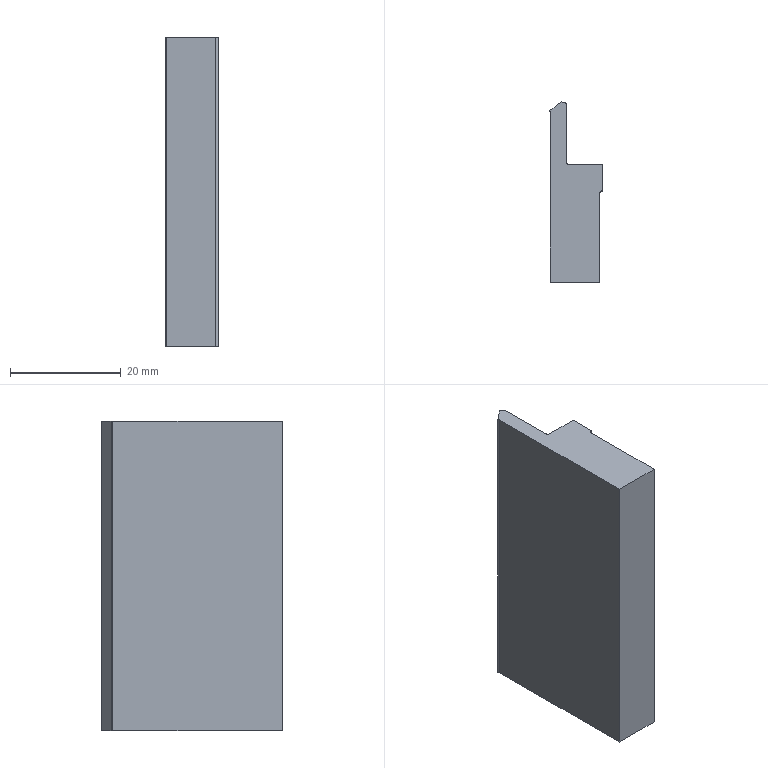Part | NX | features BREP 2 | 2 solids | 28 faces | box 9.487 x 32.71 x 56 mm | volume 24904 mm3 | plane 18 | cylinder 10 | commonest cylinder face diameters 1 x10
STEP:
#1=CARTESIAN_POINT('',(4.221,-0.3316,-4.));
#2=VERTEX_POINT('',#1);
#3=CARTESIAN_POINT('',(4.221,-0.3316,52.));
#4=VERTEX_POINT('',#3);
#5=CARTESIAN_POINT('',(4.221,-0.3316,0.));
#6=DIRECTION('',(0.,0.,1.));
#7=VECTOR('',#6,1000.);
#8=LINE('',#5,#7);
#9=EDGE_CURVE('',#2,#4,#8,.T.);
#10=ORIENTED_EDGE('',*,*,#9,.T.);
#11=CARTESIAN_POINT('',(4.221,-16.355,52.));
#12=VERTEX_POINT('',#11);
#13=CARTESIAN_POINT('',(4.221,10.146,52.));
#14=DIRECTION('',(0.,1.,0.));
#15=VECTOR('',#14,1000.);
#16=LINE('',#13,#15);
#17=EDGE_CURVE('',#12,#4,#16,.T.);
#18=ORIENTED_EDGE('',*,*,#17,.F.);
#19=CARTESIAN_POINT('',(4.221,-16.355,-4.));
#20=VERTEX_POINT('',#19);
#21=CARTESIAN_POINT('',(4.221,-16.355,0.));
#22=DIRECTION('',(0.,0.,1.));
#23=VECTOR('',#22,1000.);
#24=LINE('',#21,#23);
#25=EDGE_CURVE('',#20,#12,#24,.T.);
#26=ORIENTED_EDGE('',*,*,#25,.F.);
#27=CARTESIAN_POINT('',(4.221,10.146,-4.));
#28=DIRECTION('',(0.,1.,0.));
#29=VECTOR('',#28,1000.);
#30=LINE('',#27,#29);
#31=EDGE_CURVE('',#20,#2,#30,.T.);
#32=ORIENTED_EDGE('',*,*,#31,.T.);
#33=EDGE_LOOP('',(#10,#18,#26,#32));
#34=FACE_BOUND('',#33,.T.);
#35=CARTESIAN_POINT('',(4.221,-0.3316,0.));
#36=DIRECTION('',(-1.,0.,0.));
#37=DIRECTION('',(0.,1.,0.));
#38=AXIS2_PLACEMENT_3D('',#35,#36,#37);
#39=PLANE('',#38);
#40=ADVANCED_FACE('',(#34),#39,.F.);
#41=ORIENTED_EDGE('',*,*,#25,.T.);
#42=CARTESIAN_POINT('',(-4.656,-16.355,52.));
#43=VERTEX_POINT('',#42);
#44=CARTESIAN_POINT('',(13.794,-16.355,52.));
#45=DIRECTION('',(1.,0.,0.));
#46=VECTOR('',#45,1000.);
#47=LINE('',#44,#46);
#48=EDGE_CURVE('',#43,#12,#47,.T.);
#49=ORIENTED_EDGE('',*,*,#48,.F.);
#50=CARTESIAN_POINT('',(-4.656,-16.355,-4.));
#51=VERTEX_POINT('',#50);
#52=CARTESIAN_POINT('',(-4.656,-16.355,0.));
#53=DIRECTION('',(0.,0.,1.));
#54=VECTOR('',#53,1000.);
#55=LINE('',#52,#54);
#56=EDGE_CURVE('',#51,#43,#55,.T.);
#57=ORIENTED_EDGE('',*,*,#56,.F.);
#58=CARTESIAN_POINT('',(13.794,-16.355,-4.));
#59=DIRECTION('',(1.,0.,0.));
#60=VECTOR('',#59,1000.);
#61=LINE('',#58,#60);
#62=EDGE_CURVE('',#51,#20,#61,.T.);
#63=ORIENTED_EDGE('',*,*,#62,.T.);
#64=EDGE_LOOP('',(#41,#49,#57,#63));
#65=FACE_BOUND('',#64,.T.);
#66=CARTESIAN_POINT('',(-4.656,-16.355,0.));
#67=DIRECTION('',(0.,-1.,0.));
#68=DIRECTION('',(-1.,0.,0.));
#69=AXIS2_PLACEMENT_3D('',#66,#67,#68);
#70=PLANE('',#69);
#71=ADVANCED_FACE('',(#65),#70,.T.);
#72=ORIENTED_EDGE('',*,*,#56,.T.);
#73=CARTESIAN_POINT('',(-4.656,14.338,52.));
#74=VERTEX_POINT('',#73);
#75=CARTESIAN_POINT('',(-4.656,10.146,52.));
#76=DIRECTION('',(0.,-1.,0.));
#77=VECTOR('',#76,1000.);
#78=LINE('',#75,#77);
#79=EDGE_CURVE('',#74,#43,#78,.T.);
#80=ORIENTED_EDGE('',*,*,#79,.F.);
#81=CARTESIAN_POINT('',(-4.656,14.338,-4.));
#82=VERTEX_POINT('',#81);
#83=CARTESIAN_POINT('',(-4.656,14.338,0.));
#84=DIRECTION('',(0.,0.,1.));
#85=VECTOR('',#84,1000.);
#86=LINE('',#83,#85);
#87=EDGE_CURVE('',#82,#74,#86,.T.);
#88=ORIENTED_EDGE('',*,*,#87,.F.);
#89=CARTESIAN_POINT('',(-4.656,10.146,-4.));
#90=DIRECTION('',(0.,-1.,0.));
#91=VECTOR('',#90,1000.);
#92=LINE('',#89,#91);
#93=EDGE_CURVE('',#82,#51,#92,.T.);
#94=ORIENTED_EDGE('',*,*,#93,.T.);
#95=EDGE_LOOP('',(#72,#80,#88,#94));
#96=FACE_BOUND('',#95,.T.);
#97=CARTESIAN_POINT('',(-4.656,-17.855,0.));
#98=DIRECTION('',(1.,0.,0.));
#99=DIRECTION('',(0.,-1.,0.));
#100=AXIS2_PLACEMENT_3D('',#97,#98,#99);
#101=PLANE('',#100);
#102=ADVANCED_FACE('',(#96),#101,.F.);
#103=ORIENTED_EDGE('',*,*,#87,.T.);
#104=CARTESIAN_POINT('',(-4.766,14.651,52.));
#105=VERTEX_POINT('',#104);
#106=CARTESIAN_POINT('',(-5.156,14.338,52.));
#107=DIRECTION('',(0.,0.,-1.));
#108=DIRECTION('',(1.,0.,0.));
#109=AXIS2_PLACEMENT_3D('',#106,#107,#108);
#110=CIRCLE('',#109,0.5);
#111=EDGE_CURVE('',#105,#74,#110,.T.);
#112=ORIENTED_EDGE('',*,*,#111,.F.);
#113=CARTESIAN_POINT('',(-4.766,14.651,-4.));
#114=VERTEX_POINT('',#113);
#115=CARTESIAN_POINT('',(-4.766,14.651,0.));
#116=DIRECTION('',(0.,0.,1.));
#117=VECTOR('',#116,1000.);
#118=LINE('',#115,#117);
#119=EDGE_CURVE('',#114,#105,#118,.T.);
#120=ORIENTED_EDGE('',*,*,#119,.F.);
#121=CARTESIAN_POINT('',(-5.156,14.338,-4.));
#122=DIRECTION('',(0.,0.,-1.));
#123=DIRECTION('',(1.,0.,0.));
#124=AXIS2_PLACEMENT_3D('',#121,#122,#123);
#125=CIRCLE('',#124,0.5);
#126=EDGE_CURVE('',#114,#82,#125,.T.);
#127=ORIENTED_EDGE('',*,*,#126,.T.);
#128=EDGE_LOOP('',(#103,#112,#120,#127));
#129=FACE_BOUND('',#128,.T.);
#130=CARTESIAN_POINT('',(-5.156,14.338,0.));
#131=DIRECTION('',(0.,0.,1.));
#132=DIRECTION('',(-1.,0.,0.));
#133=AXIS2_PLACEMENT_3D('',#130,#131,#132);
#134=CYLINDRICAL_SURFACE('',#133,0.5);
#135=ADVANCED_FACE('',(#129),#134,.F.);
#136=ORIENTED_EDGE('',*,*,#119,.T.);
#137=CARTESIAN_POINT('',(-2.645,16.355,52.));
#138=VERTEX_POINT('',#137);
#139=CARTESIAN_POINT('',(-5.156,14.338,52.));
#140=DIRECTION('',(-0.7795,-0.6264,0.));
#141=VECTOR('',#140,1000.);
#142=LINE('',#139,#141);
#143=EDGE_CURVE('',#138,#105,#142,.T.);
#144=ORIENTED_EDGE('',*,*,#143,.F.);
#145=CARTESIAN_POINT('',(-2.645,16.355,-4.));
#146=VERTEX_POINT('',#145);
#147=CARTESIAN_POINT('',(-2.645,16.355,0.));
#148=DIRECTION('',(0.,0.,1.));
#149=VECTOR('',#148,1000.);
#150=LINE('',#147,#149);
#151=EDGE_CURVE('',#146,#138,#150,.T.);
#152=ORIENTED_EDGE('',*,*,#151,.F.);
#153=CARTESIAN_POINT('',(-5.156,14.338,-4.));
#154=DIRECTION('',(-0.7795,-0.6264,0.));
#155=VECTOR('',#154,1000.);
#156=LINE('',#153,#155);
#157=EDGE_CURVE('',#146,#114,#156,.T.);
#158=ORIENTED_EDGE('',*,*,#157,.T.);
#159=EDGE_LOOP('',(#136,#144,#152,#158));
#160=FACE_BOUND('',#159,.T.);
#161=CARTESIAN_POINT('',(-5.156,14.338,0.));
#162=DIRECTION('',(0.6264,-0.7795,0.));
#163=DIRECTION('',(-0.7795,-0.6264,0.));
#164=AXIS2_PLACEMENT_3D('',#161,#162,#163);
#165=PLANE('',#164);
#166=ADVANCED_FACE('',(#160),#165,.F.);
#167=ORIENTED_EDGE('',*,*,#151,.T.);
#168=CARTESIAN_POINT('',(-2.256,16.168,52.));
#169=VERTEX_POINT('',#168);
#170=CARTESIAN_POINT('',(-2.256,16.668,52.));
#171=DIRECTION('',(0.,0.,-1.));
#172=DIRECTION('',(1.,0.,0.));
#173=AXIS2_PLACEMENT_3D('',#170,#171,#172);
#174=CIRCLE('',#173,0.5);
#175=EDGE_CURVE('',#169,#138,#174,.T.);
#176=ORIENTED_EDGE('',*,*,#175,.F.);
#177=CARTESIAN_POINT('',(-2.256,16.168,-4.));
#178=VERTEX_POINT('',#177);
#179=CARTESIAN_POINT('',(-2.256,16.168,0.));
#180=DIRECTION('',(0.,0.,1.));
#181=VECTOR('',#180,1000.);
#182=LINE('',#179,#181);
#183=EDGE_CURVE('',#178,#169,#182,.T.);
#184=ORIENTED_EDGE('',*,*,#183,.F.);
#185=CARTESIAN_POINT('',(-2.256,16.668,-4.));
#186=DIRECTION('',(0.,0.,-1.));
#187=DIRECTION('',(1.,0.,0.));
#188=AXIS2_PLACEMENT_3D('',#185,#186,#187);
#189=CIRCLE('',#188,0.5);
#190=EDGE_CURVE('',#178,#146,#189,.T.);
#191=ORIENTED_EDGE('',*,*,#190,.T.);
#192=EDGE_LOOP('',(#167,#176,#184,#191));
#193=FACE_BOUND('',#192,.T.);
#194=CARTESIAN_POINT('',(-2.256,16.668,0.));
#195=DIRECTION('',(0.,0.,1.));
#196=DIRECTION('',(-1.,0.,0.));
#197=AXIS2_PLACEMENT_3D('',#194,#195,#196);
#198=CYLINDRICAL_SURFACE('',#197,0.5);
#199=ADVANCED_FACE('',(#193),#198,.F.);
#200=ORIENTED_EDGE('',*,*,#183,.T.);
#201=CARTESIAN_POINT('',(-1.756,15.668,52.));
#202=VERTEX_POINT('',#201);
#203=CARTESIAN_POINT('',(-2.256,15.668,52.));
#204=DIRECTION('',(0.,0.,1.));
#205=DIRECTION('',(1.,0.,0.));
#206=AXIS2_PLACEMENT_3D('',#203,#204,#205);
#207=CIRCLE('',#206,0.5);
#208=EDGE_CURVE('',#202,#169,#207,.T.);
#209=ORIENTED_EDGE('',*,*,#208,.F.);
#210=CARTESIAN_POINT('',(-1.756,15.668,-4.));
#211=VERTEX_POINT('',#210);
#212=CARTESIAN_POINT('',(-1.756,15.668,0.));
#213=DIRECTION('',(0.,0.,1.));
#214=VECTOR('',#213,1000.);
#215=LINE('',#212,#214);
#216=EDGE_CURVE('',#211,#202,#215,.T.);
#217=ORIENTED_EDGE('',*,*,#216,.F.);
#218=CARTESIAN_POINT('',(-2.256,15.668,-4.));
#219=DIRECTION('',(0.,0.,1.));
#220=DIRECTION('',(1.,0.,0.));
#221=AXIS2_PLACEMENT_3D('',#218,#219,#220);
#222=CIRCLE('',#221,0.5);
#223=EDGE_CURVE('',#211,#178,#222,.T.);
#224=ORIENTED_EDGE('',*,*,#223,.T.);
#225=EDGE_LOOP('',(#200,#209,#217,#224));
#226=FACE_BOUND('',#225,.T.);
#227=CARTESIAN_POINT('',(-2.256,15.668,0.));
#228=DIRECTION('',(0.,0.,1.));
#229=DIRECTION('',(-1.,0.,0.));
#230=AXIS2_PLACEMENT_3D('',#227,#228,#229);
#231=CYLINDRICAL_SURFACE('',#230,0.5);
#232=ADVANCED_FACE('',(#226),#231,.T.);
#233=ORIENTED_EDGE('',*,*,#216,.T.);
#234=CARTESIAN_POINT('',(-1.756,5.368,52.));
#235=VERTEX_POINT('',#234);
#236=CARTESIAN_POINT('',(-1.756,10.146,52.));
#237=DIRECTION('',(0.,1.,0.));
#238=VECTOR('',#237,1000.);
#239=LINE('',#236,#238);
#240=EDGE_CURVE('',#235,#202,#239,.T.);
#241=ORIENTED_EDGE('',*,*,#240,.F.);
#242=CARTESIAN_POINT('',(-1.756,5.368,-4.));
#243=VERTEX_POINT('',#242);
#244=CARTESIAN_POINT('',(-1.756,5.368,0.));
#245=DIRECTION('',(0.,0.,1.));
#246=VECTOR('',#245,1000.);
#247=LINE('',#244,#246);
#248=EDGE_CURVE('',#243,#235,#247,.T.);
#249=ORIENTED_EDGE('',*,*,#248,.F.);
#250=CARTESIAN_POINT('',(-1.756,10.146,-4.));
#251=DIRECTION('',(0.,1.,0.));
#252=VECTOR('',#251,1000.);
#253=LINE('',#250,#252);
#254=EDGE_CURVE('',#243,#211,#253,.T.);
#255=ORIENTED_EDGE('',*,*,#254,.T.);
#256=EDGE_LOOP('',(#233,#241,#249,#255));
#257=FACE_BOUND('',#256,.T.);
#258=CARTESIAN_POINT('',(-1.756,15.668,0.));
#259=DIRECTION('',(-1.,0.,0.));
#260=DIRECTION('',(0.,1.,0.));
#261=AXIS2_PLACEMENT_3D('',#258,#259,#260);
#262=PLANE('',#261);
#263=ADVANCED_FACE('',(#257),#262,.F.);
#264=ORIENTED_EDGE('',*,*,#248,.T.);
#265=CARTESIAN_POINT('',(-1.256,4.868,52.));
#266=VERTEX_POINT('',#265);
#267=CARTESIAN_POINT('',(-1.256,5.368,52.));
#268=DIRECTION('',(0.,0.,-1.));
#269=DIRECTION('',(1.,0.,0.));
#270=AXIS2_PLACEMENT_3D('',#267,#268,#269);
#271=CIRCLE('',#270,0.5);
#272=EDGE_CURVE('',#266,#235,#271,.T.);
#273=ORIENTED_EDGE('',*,*,#272,.F.);
#274=CARTESIAN_POINT('',(-1.256,4.868,-4.));
#275=VERTEX_POINT('',#274);
#276=CARTESIAN_POINT('',(-1.256,4.868,0.));
#277=DIRECTION('',(0.,0.,1.));
#278=VECTOR('',#277,1000.);
#279=LINE('',#276,#278);
#280=EDGE_CURVE('',#275,#266,#279,.T.);
#281=ORIENTED_EDGE('',*,*,#280,.F.);
#282=CARTESIAN_POINT('',(-1.256,5.368,-4.));
#283=DIRECTION('',(0.,0.,-1.));
#284=DIRECTION('',(1.,0.,0.));
#285=AXIS2_PLACEMENT_3D('',#282,#283,#284);
#286=CIRCLE('',#285,0.5);
#287=EDGE_CURVE('',#275,#243,#286,.T.);
#288=ORIENTED_EDGE('',*,*,#287,.T.);
#289=EDGE_LOOP('',(#264,#273,#281,#288));
#290=FACE_BOUND('',#289,.T.);
#291=CARTESIAN_POINT('',(-1.256,5.368,0.));
#292=DIRECTION('',(0.,0.,1.));
#293=DIRECTION('',(-1.,0.,0.));
#294=AXIS2_PLACEMENT_3D('',#291,#292,#293);
#295=CYLINDRICAL_SURFACE('',#294,0.5);
#296=ADVANCED_FACE('',(#290),#295,.F.);
#297=ORIENTED_EDGE('',*,*,#280,.T.);
#298=CARTESIAN_POINT('',(4.721,4.868,52.));
#299=VERTEX_POINT('',#298);
#300=CARTESIAN_POINT('',(13.794,4.868,52.));
#301=DIRECTION('',(-1.,0.,0.));
#302=VECTOR('',#301,1000.);
#303=LINE('',#300,#302);
#304=EDGE_CURVE('',#299,#266,#303,.T.);
#305=ORIENTED_EDGE('',*,*,#304,.F.);
#306=CARTESIAN_POINT('',(4.721,4.868,-4.));
#307=VERTEX_POINT('',#306);
#308=CARTESIAN_POINT('',(4.721,4.868,0.));
#309=DIRECTION('',(0.,0.,1.));
#310=VECTOR('',#309,1000.);
#311=LINE('',#308,#310);
#312=EDGE_CURVE('',#307,#299,#311,.T.);
#313=ORIENTED_EDGE('',*,*,#312,.F.);
#314=CARTESIAN_POINT('',(13.794,4.868,-4.));
#315=DIRECTION('',(-1.,0.,0.));
#316=VECTOR('',#315,1000.);
#317=LINE('',#314,#316);
#318=EDGE_CURVE('',#307,#275,#317,.T.);
#319=ORIENTED_EDGE('',*,*,#318,.T.);
#320=EDGE_LOOP('',(#297,#305,#313,#319));
#321=FACE_BOUND('',#320,.T.);
#322=CARTESIAN_POINT('',(-1.256,4.868,0.));
#323=DIRECTION('',(0.,-1.,0.));
#324=DIRECTION('',(-1.,0.,0.));
#325=AXIS2_PLACEMENT_3D('',#322,#323,#324);
#326=PLANE('',#325);
#327=ADVANCED_FACE('',(#321),#326,.F.);
#328=ORIENTED_EDGE('',*,*,#312,.T.);
#329=CARTESIAN_POINT('',(4.721,0.1684,52.));
#330=VERTEX_POINT('',#329);
#331=CARTESIAN_POINT('',(4.721,10.146,52.));
#332=DIRECTION('',(0.,1.,0.));
#333=VECTOR('',#332,1000.);
#334=LINE('',#331,#333);
#335=EDGE_CURVE('',#330,#299,#334,.T.);
#336=ORIENTED_EDGE('',*,*,#335,.F.);
#337=CARTESIAN_POINT('',(4.721,0.1684,-4.));
#338=VERTEX_POINT('',#337);
#339=CARTESIAN_POINT('',(4.721,0.1684,0.));
#340=DIRECTION('',(0.,0.,1.));
#341=VECTOR('',#340,1000.);
#342=LINE('',#339,#341);
#343=EDGE_CURVE('',#338,#330,#342,.T.);
#344=ORIENTED_EDGE('',*,*,#343,.F.);
#345=CARTESIAN_POINT('',(4.721,10.146,-4.));
#346=DIRECTION('',(0.,1.,0.));
#347=VECTOR('',#346,1000.);
#348=LINE('',#345,#347);
#349=EDGE_CURVE('',#338,#307,#348,.T.);
#350=ORIENTED_EDGE('',*,*,#349,.T.);
#351=EDGE_LOOP('',(#328,#336,#344,#350));
#352=FACE_BOUND('',#351,.T.);
#353=CARTESIAN_POINT('',(4.721,10.146,0.));
#354=DIRECTION('',(-1.,0.,0.));
#355=DIRECTION('',(0.,1.,0.));
#356=AXIS2_PLACEMENT_3D('',#353,#354,#355);
#357=PLANE('',#356);
#358=ADVANCED_FACE('',(#352),#357,.F.);
#359=CARTESIAN_POINT('',(4.721,-0.3316,-4.));
#360=DIRECTION('',(0.,0.,-1.));
#361=DIRECTION('',(1.,0.,0.));
#362=AXIS2_PLACEMENT_3D('',#359,#360,#361);
#363=CIRCLE('',#362,0.5);
#364=EDGE_CURVE('',#2,#338,#363,.T.);
#365=ORIENTED_EDGE('',*,*,#364,.T.);
#366=ORIENTED_EDGE('',*,*,#343,.T.);
#367=CARTESIAN_POINT('',(4.721,-0.3316,52.));
#368=DIRECTION('',(0.,0.,-1.));
#369=DIRECTION('',(1.,0.,0.));
#370=AXIS2_PLACEMENT_3D('',#367,#368,#369);
#371=CIRCLE('',#370,0.5);
#372=EDGE_CURVE('',#4,#330,#371,.T.);
#373=ORIENTED_EDGE('',*,*,#372,.F.);
#374=ORIENTED_EDGE('',*,*,#9,.F.);
#375=EDGE_LOOP('',(#365,#366,#373,#374));
#376=FACE_BOUND('',#375,.T.);
#377=CARTESIAN_POINT('',(4.721,-0.3316,0.));
#378=DIRECTION('',(0.,0.,1.));
#379=DIRECTION('',(-1.,0.,0.));
#380=AXIS2_PLACEMENT_3D('',#377,#378,#379);
#381=CYLINDRICAL_SURFACE('',#380,0.5);
#382=ADVANCED_FACE('',(#376),#381,.F.);
#383=ORIENTED_EDGE('',*,*,#335,.T.);
#384=ORIENTED_EDGE('',*,*,#304,.T.);
#385=ORIENTED_EDGE('',*,*,#272,.T.);
#386=ORIENTED_EDGE('',*,*,#240,.T.);
#387=ORIENTED_EDGE('',*,*,#208,.T.);
#388=ORIENTED_EDGE('',*,*,#175,.T.);
#389=ORIENTED_EDGE('',*,*,#143,.T.);
#390=ORIENTED_EDGE('',*,*,#111,.T.);
#391=ORIENTED_EDGE('',*,*,#79,.T.);
#392=ORIENTED_EDGE('',*,*,#48,.T.);
#393=ORIENTED_EDGE('',*,*,#17,.T.);
#394=ORIENTED_EDGE('',*,*,#372,.T.);
#395=EDGE_LOOP('',(#383,#384,#385,#386,#387,#388,#389,#390,#391,#392,#393,#394));
#396=FACE_BOUND('',#395,.T.);
#397=CARTESIAN_POINT('',(13.794,10.146,52.));
#398=DIRECTION('',(0.,0.,1.));
#399=DIRECTION('',(-1.,0.,0.));
#400=AXIS2_PLACEMENT_3D('',#397,#398,#399);
#401=PLANE('',#400);
#402=ADVANCED_FACE('',(#396),#401,.T.);
#403=ORIENTED_EDGE('',*,*,#349,.F.);
#404=ORIENTED_EDGE('',*,*,#364,.F.);
#405=ORIENTED_EDGE('',*,*,#31,.F.);
#406=ORIENTED_EDGE('',*,*,#62,.F.);
#407=ORIENTED_EDGE('',*,*,#93,.F.);
#408=ORIENTED_EDGE('',*,*,#126,.F.);
#409=ORIENTED_EDGE('',*,*,#157,.F.);
#410=ORIENTED_EDGE('',*,*,#190,.F.);
#411=ORIENTED_EDGE('',*,*,#223,.F.);
#412=ORIENTED_EDGE('',*,*,#254,.F.);
#413=ORIENTED_EDGE('',*,*,#287,.F.);
#414=ORIENTED_EDGE('',*,*,#318,.F.);
#415=EDGE_LOOP('',(#403,#404,#405,#406,#407,#408,#409,#410,#411,#412,#413,#414));
#416=FACE_BOUND('',#415,.T.);
#417=CARTESIAN_POINT('',(13.794,10.146,-4.));
#418=DIRECTION('',(0.,0.,1.));
#419=DIRECTION('',(-1.,0.,0.));
#420=AXIS2_PLACEMENT_3D('',#417,#418,#419);
#421=PLANE('',#420);
#422=ADVANCED_FACE('',(#416),#421,.F.);
#423=CLOSED_SHELL('',(#40,#71,#102,#135,#166,#199,#232,#263,#296,#327,#358,#382,#402,#422));
#424=MANIFOLD_SOLID_BREP('',#423);
#425=CARTESIAN_POINT('',(4.221,-0.3316,-4.));
#426=VERTEX_POINT('',#425);
#427=CARTESIAN_POINT('',(4.221,-0.3316,52.));
#428=VERTEX_POINT('',#427);
#429=CARTESIAN_POINT('',(4.221,-0.3316,0.));
#430=DIRECTION('',(0.,0.,1.));
#431=VECTOR('',#430,1000.);
#432=LINE('',#429,#431);
#433=EDGE_CURVE('',#426,#428,#432,.T.);
#434=ORIENTED_EDGE('',*,*,#433,.T.);
#435=CARTESIAN_POINT('',(4.221,-16.355,52.));
#436=VERTEX_POINT('',#435);
#437=CARTESIAN_POINT('',(4.221,10.146,52.));
#438=DIRECTION('',(0.,1.,0.));
#439=VECTOR('',#438,1000.);
#440=LINE('',#437,#439);
#441=EDGE_CURVE('',#436,#428,#440,.T.);
#442=ORIENTED_EDGE('',*,*,#441,.F.);
#443=CARTESIAN_POINT('',(4.221,-16.355,-4.));
#444=VERTEX_POINT('',#443);
#445=CARTESIAN_POINT('',(4.221,-16.355,0.));
#446=DIRECTION('',(0.,0.,1.));
#447=VECTOR('',#446,1000.);
#448=LINE('',#445,#447);
#449=EDGE_CURVE('',#444,#436,#448,.T.);
#450=ORIENTED_EDGE('',*,*,#449,.F.);
#451=CARTESIAN_POINT('',(4.221,10.146,-4.));
#452=DIRECTION('',(0.,1.,0.));
#453=VECTOR('',#452,1000.);
#454=LINE('',#451,#453);
#455=EDGE_CURVE('',#444,#426,#454,.T.);
#456=ORIENTED_EDGE('',*,*,#455,.T.);
#457=EDGE_LOOP('',(#434,#442,#450,#456));
#458=FACE_BOUND('',#457,.T.);
#459=CARTESIAN_POINT('',(4.221,-0.3316,0.));
#460=DIRECTION('',(-1.,0.,0.));
#461=DIRECTION('',(0.,1.,0.));
#462=AXIS2_PLACEMENT_3D('',#459,#460,#461);
#463=PLANE('',#462);
#464=ADVANCED_FACE('',(#458),#463,.F.);
#465=ORIENTED_EDGE('',*,*,#449,.T.);
#466=CARTESIAN_POINT('',(-4.656,-16.355,52.));
#467=VERTEX_POINT('',#466);
#468=CARTESIAN_POINT('',(13.794,-16.355,52.));
#469=DIRECTION('',(1.,0.,0.));
#470=VECTOR('',#469,1000.);
#471=LINE('',#468,#470);
#472=EDGE_CURVE('',#467,#436,#471,.T.);
#473=ORIENTED_EDGE('',*,*,#472,.F.);
#474=CARTESIAN_POINT('',(-4.656,-16.355,-4.));
#475=VERTEX_POINT('',#474);
#476=CARTESIAN_POINT('',(-4.656,-16.355,0.));
#477=DIRECTION('',(0.,0.,1.));
#478=VECTOR('',#477,1000.);
#479=LINE('',#476,#478);
#480=EDGE_CURVE('',#475,#467,#479,.T.);
#481=ORIENTED_EDGE('',*,*,#480,.F.);
#482=CARTESIAN_POINT('',(13.794,-16.355,-4.));
#483=DIRECTION('',(1.,0.,0.));
#484=VECTOR('',#483,1000.);
#485=LINE('',#482,#484);
#486=EDGE_CURVE('',#475,#444,#485,.T.);
#487=ORIENTED_EDGE('',*,*,#486,.T.);
#488=EDGE_LOOP('',(#465,#473,#481,#487));
#489=FACE_BOUND('',#488,.T.);
#490=CARTESIAN_POINT('',(-4.656,-16.355,0.));
#491=DIRECTION('',(0.,-1.,0.));
#492=DIRECTION('',(-1.,0.,0.));
#493=AXIS2_PLACEMENT_3D('',#490,#491,#492);
#494=PLANE('',#493);
#495=ADVANCED_FACE('',(#489),#494,.T.);
#496=ORIENTED_EDGE('',*,*,#480,.T.);
#497=CARTESIAN_POINT('',(-4.656,14.338,52.));
#498=VERTEX_POINT('',#497);
#499=CARTESIAN_POINT('',(-4.656,10.146,52.));
#500=DIRECTION('',(0.,-1.,0.));
#501=VECTOR('',#500,1000.);
#502=LINE('',#499,#501);
#503=EDGE_CURVE('',#498,#467,#502,.T.);
#504=ORIENTED_EDGE('',*,*,#503,.F.);
#505=CARTESIAN_POINT('',(-4.656,14.338,-4.));
#506=VERTEX_POINT('',#505);
#507=CARTESIAN_POINT('',(-4.656,14.338,0.));
#508=DIRECTION('',(0.,0.,1.));
#509=VECTOR('',#508,1000.);
#510=LINE('',#507,#509);
#511=EDGE_CURVE('',#506,#498,#510,.T.);
#512=ORIENTED_EDGE('',*,*,#511,.F.);
#513=CARTESIAN_POINT('',(-4.656,10.146,-4.));
#514=DIRECTION('',(0.,-1.,0.));
#515=VECTOR('',#514,1000.);
#516=LINE('',#513,#515);
#517=EDGE_CURVE('',#506,#475,#516,.T.);
#518=ORIENTED_EDGE('',*,*,#517,.T.);
#519=EDGE_LOOP('',(#496,#504,#512,#518));
#520=FACE_BOUND('',#519,.T.);
#521=CARTESIAN_POINT('',(-4.656,-17.855,0.));
#522=DIRECTION('',(1.,0.,0.));
#523=DIRECTION('',(0.,-1.,0.));
#524=AXIS2_PLACEMENT_3D('',#521,#522,#523);
#525=PLANE('',#524);
#526=ADVANCED_FACE('',(#520),#525,.F.);
#527=ORIENTED_EDGE('',*,*,#511,.T.);
#528=CARTESIAN_POINT('',(-4.766,14.651,52.));
#529=VERTEX_POINT('',#528);
#530=CARTESIAN_POINT('',(-5.156,14.338,52.));
#531=DIRECTION('',(0.,0.,-1.));
#532=DIRECTION('',(1.,0.,0.));
#533=AXIS2_PLACEMENT_3D('',#530,#531,#532);
#534=CIRCLE('',#533,0.5);
#535=EDGE_CURVE('',#529,#498,#534,.T.);
#536=ORIENTED_EDGE('',*,*,#535,.F.);
#537=CARTESIAN_POINT('',(-4.766,14.651,-4.));
#538=VERTEX_POINT('',#537);
#539=CARTESIAN_POINT('',(-4.766,14.651,0.));
#540=DIRECTION('',(0.,0.,1.));
#541=VECTOR('',#540,1000.);
#542=LINE('',#539,#541);
#543=EDGE_CURVE('',#538,#529,#542,.T.);
#544=ORIENTED_EDGE('',*,*,#543,.F.);
#545=CARTESIAN_POINT('',(-5.156,14.338,-4.));
#546=DIRECTION('',(0.,0.,-1.));
#547=DIRECTION('',(1.,0.,0.));
#548=AXIS2_PLACEMENT_3D('',#545,#546,#547);
#549=CIRCLE('',#548,0.5);
#550=EDGE_CURVE('',#538,#506,#549,.T.);
#551=ORIENTED_EDGE('',*,*,#550,.T.);
#552=EDGE_LOOP('',(#527,#536,#544,#551));
#553=FACE_BOUND('',#552,.T.);
#554=CARTESIAN_POINT('',(-5.156,14.338,0.));
#555=DIRECTION('',(0.,0.,1.));
#556=DIRECTION('',(-1.,0.,0.));
#557=AXIS2_PLACEMENT_3D('',#554,#555,#556);
#558=CYLINDRICAL_SURFACE('',#557,0.5);
#559=ADVANCED_FACE('',(#553),#558,.F.);
#560=ORIENTED_EDGE('',*,*,#543,.T.);
#561=CARTESIAN_POINT('',(-2.645,16.355,52.));
#562=VERTEX_POINT('',#561);
#563=CARTESIAN_POINT('',(-5.156,14.338,52.));
#564=DIRECTION('',(-0.7795,-0.6264,0.));
#565=VECTOR('',#564,1000.);
#566=LINE('',#563,#565);
#567=EDGE_CURVE('',#562,#529,#566,.T.);
#568=ORIENTED_EDGE('',*,*,#567,.F.);
#569=CARTESIAN_POINT('',(-2.645,16.355,-4.));
#570=VERTEX_POINT('',#569);
#571=CARTESIAN_POINT('',(-2.645,16.355,0.));
#572=DIRECTION('',(0.,0.,1.));
#573=VECTOR('',#572,1000.);
#574=LINE('',#571,#573);
#575=EDGE_CURVE('',#570,#562,#574,.T.);
#576=ORIENTED_EDGE('',*,*,#575,.F.);
#577=CARTESIAN_POINT('',(-5.156,14.338,-4.));
#578=DIRECTION('',(-0.7795,-0.6264,0.));
#579=VECTOR('',#578,1000.);
#580=LINE('',#577,#579);
#581=EDGE_CURVE('',#570,#538,#580,.T.);
#582=ORIENTED_EDGE('',*,*,#581,.T.);
#583=EDGE_LOOP('',(#560,#568,#576,#582));
#584=FACE_BOUND('',#583,.T.);
#585=CARTESIAN_POINT('',(-5.156,14.338,0.));
#586=DIRECTION('',(0.6264,-0.7795,0.));
#587=DIRECTION('',(-0.7795,-0.6264,0.));
#588=AXIS2_PLACEMENT_3D('',#585,#586,#587);
#589=PLANE('',#588);
#590=ADVANCED_FACE('',(#584),#589,.F.);
#591=ORIENTED_EDGE('',*,*,#575,.T.);
#592=CARTESIAN_POINT('',(-2.256,16.168,52.));
#593=VERTEX_POINT('',#592);
#594=CARTESIAN_POINT('',(-2.256,16.668,52.));
#595=DIRECTION('',(0.,0.,-1.));
#596=DIRECTION('',(1.,0.,0.));
#597=AXIS2_PLACEMENT_3D('',#594,#595,#596);
#598=CIRCLE('',#597,0.5);
#599=EDGE_CURVE('',#593,#562,#598,.T.);
#600=ORIENTED_EDGE('',*,*,#599,.F.);
#601=CARTESIAN_POINT('',(-2.256,16.168,-4.));
#602=VERTEX_POINT('',#601);
#603=CARTESIAN_POINT('',(-2.256,16.168,0.));
#604=DIRECTION('',(0.,0.,1.));
#605=VECTOR('',#604,1000.);
#606=LINE('',#603,#605);
#607=EDGE_CURVE('',#602,#593,#606,.T.);
#608=ORIENTED_EDGE('',*,*,#607,.F.);
#609=CARTESIAN_POINT('',(-2.256,16.668,-4.));
#610=DIRECTION('',(0.,0.,-1.));
#611=DIRECTION('',(1.,0.,0.));
#612=AXIS2_PLACEMENT_3D('',#609,#610,#611);
#613=CIRCLE('',#612,0.5);
#614=EDGE_CURVE('',#602,#570,#613,.T.);
#615=ORIENTED_EDGE('',*,*,#614,.T.);
#616=EDGE_LOOP('',(#591,#600,#608,#615));
#617=FACE_BOUND('',#616,.T.);
#618=CARTESIAN_POINT('',(-2.256,16.668,0.));
#619=DIRECTION('',(0.,0.,1.));
#620=DIRECTION('',(-1.,0.,0.));
#621=AXIS2_PLACEMENT_3D('',#618,#619,#620);
#622=CYLINDRICAL_SURFACE('',#621,0.5);
#623=ADVANCED_FACE('',(#617),#622,.F.);
#624=ORIENTED_EDGE('',*,*,#607,.T.);
#625=CARTESIAN_POINT('',(-1.756,15.668,52.));
#626=VERTEX_POINT('',#625);
#627=CARTESIAN_POINT('',(-2.256,15.668,52.));
#628=DIRECTION('',(0.,0.,1.));
#629=DIRECTION('',(1.,0.,0.));
#630=AXIS2_PLACEMENT_3D('',#627,#628,#629);
#631=CIRCLE('',#630,0.5);
#632=EDGE_CURVE('',#626,#593,#631,.T.);
#633=ORIENTED_EDGE('',*,*,#632,.F.);
#634=CARTESIAN_POINT('',(-1.756,15.668,-4.));
#635=VERTEX_POINT('',#634);
#636=CARTESIAN_POINT('',(-1.756,15.668,0.));
#637=DIRECTION('',(0.,0.,1.));
#638=VECTOR('',#637,1000.);
#639=LINE('',#636,#638);
#640=EDGE_CURVE('',#635,#626,#639,.T.);
#641=ORIENTED_EDGE('',*,*,#640,.F.);
#642=CARTESIAN_POINT('',(-2.256,15.668,-4.));
#643=DIRECTION('',(0.,0.,1.));
#644=DIRECTION('',(1.,0.,0.));
#645=AXIS2_PLACEMENT_3D('',#642,#643,#644);
#646=CIRCLE('',#645,0.5);
#647=EDGE_CURVE('',#635,#602,#646,.T.);
#648=ORIENTED_EDGE('',*,*,#647,.T.);
#649=EDGE_LOOP('',(#624,#633,#641,#648));
#650=FACE_BOUND('',#649,.T.);
#651=CARTESIAN_POINT('',(-2.256,15.668,0.));
#652=DIRECTION('',(0.,0.,1.));
#653=DIRECTION('',(-1.,0.,0.));
#654=AXIS2_PLACEMENT_3D('',#651,#652,#653);
#655=CYLINDRICAL_SURFACE('',#654,0.5);
#656=ADVANCED_FACE('',(#650),#655,.T.);
#657=ORIENTED_EDGE('',*,*,#640,.T.);
#658=CARTESIAN_POINT('',(-1.756,5.368,52.));
#659=VERTEX_POINT('',#658);
#660=CARTESIAN_POINT('',(-1.756,10.146,52.));
#661=DIRECTION('',(0.,1.,0.));
#662=VECTOR('',#661,1000.);
#663=LINE('',#660,#662);
#664=EDGE_CURVE('',#659,#626,#663,.T.);
#665=ORIENTED_EDGE('',*,*,#664,.F.);
#666=CARTESIAN_POINT('',(-1.756,5.368,-4.));
#667=VERTEX_POINT('',#666);
#668=CARTESIAN_POINT('',(-1.756,5.368,0.));
#669=DIRECTION('',(0.,0.,1.));
#670=VECTOR('',#669,1000.);
#671=LINE('',#668,#670);
#672=EDGE_CURVE('',#667,#659,#671,.T.);
#673=ORIENTED_EDGE('',*,*,#672,.F.);
#674=CARTESIAN_POINT('',(-1.756,10.146,-4.));
#675=DIRECTION('',(0.,1.,0.));
#676=VECTOR('',#675,1000.);
#677=LINE('',#674,#676);
#678=EDGE_CURVE('',#667,#635,#677,.T.);
#679=ORIENTED_EDGE('',*,*,#678,.T.);
#680=EDGE_LOOP('',(#657,#665,#673,#679));
#681=FACE_BOUND('',#680,.T.);
#682=CARTESIAN_POINT('',(-1.756,15.668,0.));
#683=DIRECTION('',(-1.,0.,0.));
#684=DIRECTION('',(0.,1.,0.));
#685=AXIS2_PLACEMENT_3D('',#682,#683,#684);
#686=PLANE('',#685);
#687=ADVANCED_FACE('',(#681),#686,.F.);
#688=ORIENTED_EDGE('',*,*,#672,.T.);
#689=CARTESIAN_POINT('',(-1.256,4.868,52.));
#690=VERTEX_POINT('',#689);
#691=CARTESIAN_POINT('',(-1.256,5.368,52.));
#692=DIRECTION('',(0.,0.,-1.));
#693=DIRECTION('',(1.,0.,0.));
#694=AXIS2_PLACEMENT_3D('',#691,#692,#693);
#695=CIRCLE('',#694,0.5);
#696=EDGE_CURVE('',#690,#659,#695,.T.);
#697=ORIENTED_EDGE('',*,*,#696,.F.);
#698=CARTESIAN_POINT('',(-1.256,4.868,-4.));
#699=VERTEX_POINT('',#698);
#700=CARTESIAN_POINT('',(-1.256,4.868,0.));
#701=DIRECTION('',(0.,0.,1.));
#702=VECTOR('',#701,1000.);
#703=LINE('',#700,#702);
#704=EDGE_CURVE('',#699,#690,#703,.T.);
#705=ORIENTED_EDGE('',*,*,#704,.F.);
#706=CARTESIAN_POINT('',(-1.256,5.368,-4.));
#707=DIRECTION('',(0.,0.,-1.));
#708=DIRECTION('',(1.,0.,0.));
#709=AXIS2_PLACEMENT_3D('',#706,#707,#708);
#710=CIRCLE('',#709,0.5);
#711=EDGE_CURVE('',#699,#667,#710,.T.);
#712=ORIENTED_EDGE('',*,*,#711,.T.);
#713=EDGE_LOOP('',(#688,#697,#705,#712));
#714=FACE_BOUND('',#713,.T.);
#715=CARTESIAN_POINT('',(-1.256,5.368,0.));
#716=DIRECTION('',(0.,0.,1.));
#717=DIRECTION('',(-1.,0.,0.));
#718=AXIS2_PLACEMENT_3D('',#715,#716,#717);
#719=CYLINDRICAL_SURFACE('',#718,0.5);
#720=ADVANCED_FACE('',(#714),#719,.F.);
#721=ORIENTED_EDGE('',*,*,#704,.T.);
#722=CARTESIAN_POINT('',(4.721,4.868,52.));
#723=VERTEX_POINT('',#722);
#724=CARTESIAN_POINT('',(13.794,4.868,52.));
#725=DIRECTION('',(-1.,0.,0.));
#726=VECTOR('',#725,1000.);
#727=LINE('',#724,#726);
#728=EDGE_CURVE('',#723,#690,#727,.T.);
#729=ORIENTED_EDGE('',*,*,#728,.F.);
#730=CARTESIAN_POINT('',(4.721,4.868,-4.));
#731=VERTEX_POINT('',#730);
#732=CARTESIAN_POINT('',(4.721,4.868,0.));
#733=DIRECTION('',(0.,0.,1.));
#734=VECTOR('',#733,1000.);
#735=LINE('',#732,#734);
#736=EDGE_CURVE('',#731,#723,#735,.T.);
#737=ORIENTED_EDGE('',*,*,#736,.F.);
#738=CARTESIAN_POINT('',(13.794,4.868,-4.));
#739=DIRECTION('',(-1.,0.,0.));
#740=VECTOR('',#739,1000.);
#741=LINE('',#738,#740);
#742=EDGE_CURVE('',#731,#699,#741,.T.);
#743=ORIENTED_EDGE('',*,*,#742,.T.);
#744=EDGE_LOOP('',(#721,#729,#737,#743));
#745=FACE_BOUND('',#744,.T.);
#746=CARTESIAN_POINT('',(-1.256,4.868,0.));
#747=DIRECTION('',(0.,-1.,0.));
#748=DIRECTION('',(-1.,0.,0.));
#749=AXIS2_PLACEMENT_3D('',#746,#747,#748);
#750=PLANE('',#749);
#751=ADVANCED_FACE('',(#745),#750,.F.);
#752=ORIENTED_EDGE('',*,*,#736,.T.);
#753=CARTESIAN_POINT('',(4.721,0.1684,52.));
#754=VERTEX_POINT('',#753);
#755=CARTESIAN_POINT('',(4.721,10.146,52.));
#756=DIRECTION('',(0.,1.,0.));
#757=VECTOR('',#756,1000.);
#758=LINE('',#755,#757);
#759=EDGE_CURVE('',#754,#723,#758,.T.);
#760=ORIENTED_EDGE('',*,*,#759,.F.);
#761=CARTESIAN_POINT('',(4.721,0.1684,-4.));
#762=VERTEX_POINT('',#761);
#763=CARTESIAN_POINT('',(4.721,0.1684,0.));
#764=DIRECTION('',(0.,0.,1.));
#765=VECTOR('',#764,1000.);
#766=LINE('',#763,#765);
#767=EDGE_CURVE('',#762,#754,#766,.T.);
#768=ORIENTED_EDGE('',*,*,#767,.F.);
#769=CARTESIAN_POINT('',(4.721,10.146,-4.));
#770=DIRECTION('',(0.,1.,0.));
#771=VECTOR('',#770,1000.);
#772=LINE('',#769,#771);
#773=EDGE_CURVE('',#762,#731,#772,.T.);
#774=ORIENTED_EDGE('',*,*,#773,.T.);
#775=EDGE_LOOP('',(#752,#760,#768,#774));
#776=FACE_BOUND('',#775,.T.);
#777=CARTESIAN_POINT('',(4.721,10.146,0.));
#778=DIRECTION('',(-1.,0.,0.));
#779=DIRECTION('',(0.,1.,0.));
#780=AXIS2_PLACEMENT_3D('',#777,#778,#779);
#781=PLANE('',#780);
#782=ADVANCED_FACE('',(#776),#781,.F.);
#783=CARTESIAN_POINT('',(4.721,-0.3316,-4.));
#784=DIRECTION('',(0.,0.,-1.));
#785=DIRECTION('',(1.,0.,0.));
#786=AXIS2_PLACEMENT_3D('',#783,#784,#785);
#787=CIRCLE('',#786,0.5);
#788=EDGE_CURVE('',#426,#762,#787,.T.);
#789=ORIENTED_EDGE('',*,*,#788,.T.);
#790=ORIENTED_EDGE('',*,*,#767,.T.);
#791=CARTESIAN_POINT('',(4.721,-0.3316,52.));
#792=DIRECTION('',(0.,0.,-1.));
#793=DIRECTION('',(1.,0.,0.));
#794=AXIS2_PLACEMENT_3D('',#791,#792,#793);
#795=CIRCLE('',#794,0.5);
#796=EDGE_CURVE('',#428,#754,#795,.T.);
#797=ORIENTED_EDGE('',*,*,#796,.F.);
#798=ORIENTED_EDGE('',*,*,#433,.F.);
#799=EDGE_LOOP('',(#789,#790,#797,#798));
#800=FACE_BOUND('',#799,.T.);
#801=CARTESIAN_POINT('',(4.721,-0.3316,0.));
#802=DIRECTION('',(0.,0.,1.));
#803=DIRECTION('',(-1.,0.,0.));
#804=AXIS2_PLACEMENT_3D('',#801,#802,#803);
#805=CYLINDRICAL_SURFACE('',#804,0.5);
#806=ADVANCED_FACE('',(#800),#805,.F.);
#807=ORIENTED_EDGE('',*,*,#759,.T.);
#808=ORIENTED_EDGE('',*,*,#728,.T.);
#809=ORIENTED_EDGE('',*,*,#696,.T.);
#810=ORIENTED_EDGE('',*,*,#664,.T.);
#811=ORIENTED_EDGE('',*,*,#632,.T.);
#812=ORIENTED_EDGE('',*,*,#599,.T.);
#813=ORIENTED_EDGE('',*,*,#567,.T.);
#814=ORIENTED_EDGE('',*,*,#535,.T.);
#815=ORIENTED_EDGE('',*,*,#503,.T.);
#816=ORIENTED_EDGE('',*,*,#472,.T.);
#817=ORIENTED_EDGE('',*,*,#441,.T.);
#818=ORIENTED_EDGE('',*,*,#796,.T.);
#819=EDGE_LOOP('',(#807,#808,#809,#810,#811,#812,#813,#814,#815,#816,#817,#818));
#820=FACE_BOUND('',#819,.T.);
#821=CARTESIAN_POINT('',(13.794,10.146,52.));
#822=DIRECTION('',(0.,0.,1.));
#823=DIRECTION('',(-1.,0.,0.));
#824=AXIS2_PLACEMENT_3D('',#821,#822,#823);
#825=PLANE('',#824);
#826=ADVANCED_FACE('',(#820),#825,.T.);
#827=ORIENTED_EDGE('',*,*,#773,.F.);
#828=ORIENTED_EDGE('',*,*,#788,.F.);
#829=ORIENTED_EDGE('',*,*,#455,.F.);
#830=ORIENTED_EDGE('',*,*,#486,.F.);
#831=ORIENTED_EDGE('',*,*,#517,.F.);
#832=ORIENTED_EDGE('',*,*,#550,.F.);
#833=ORIENTED_EDGE('',*,*,#581,.F.);
#834=ORIENTED_EDGE('',*,*,#614,.F.);
#835=ORIENTED_EDGE('',*,*,#647,.F.);
#836=ORIENTED_EDGE('',*,*,#678,.F.);
#837=ORIENTED_EDGE('',*,*,#711,.F.);
#838=ORIENTED_EDGE('',*,*,#742,.F.);
#839=EDGE_LOOP('',(#827,#828,#829,#830,#831,#832,#833,#834,#835,#836,#837,#838));
#840=FACE_BOUND('',#839,.T.);
#841=CARTESIAN_POINT('',(13.794,10.146,-4.));
#842=DIRECTION('',(0.,0.,1.));
#843=DIRECTION('',(-1.,0.,0.));
#844=AXIS2_PLACEMENT_3D('',#841,#842,#843);
#845=PLANE('',#844);
#846=ADVANCED_FACE('',(#840),#845,.F.);
#847=CLOSED_SHELL('',(#464,#495,#526,#559,#590,#623,#656,#687,#720,#751,#782,#806,#826,#846));
#848=MANIFOLD_SOLID_BREP('',#847);
#849=(LENGTH_UNIT()NAMED_UNIT(*)SI_UNIT(.MILLI.,.METRE.));
#850=UNCERTAINTY_MEASURE_WITH_UNIT(LENGTH_MEASURE(0.00001),#849,'','');
#851=(NAMED_UNIT(*)PLANE_ANGLE_UNIT()SI_UNIT($,.RADIAN.));
#852=(NAMED_UNIT(*)SI_UNIT($,.STERADIAN.)SOLID_ANGLE_UNIT());
#853=(GEOMETRIC_REPRESENTATION_CONTEXT(3)GLOBAL_UNCERTAINTY_ASSIGNED_CONTEXT((#850))GLOBAL_UNIT_ASSIGNED_CONTEXT((#849,#851,#852))REPRESENTATION_CONTEXT('',''));
#854=ADVANCED_BREP_SHAPE_REPRESENTATION('',(#424,#848),#853);